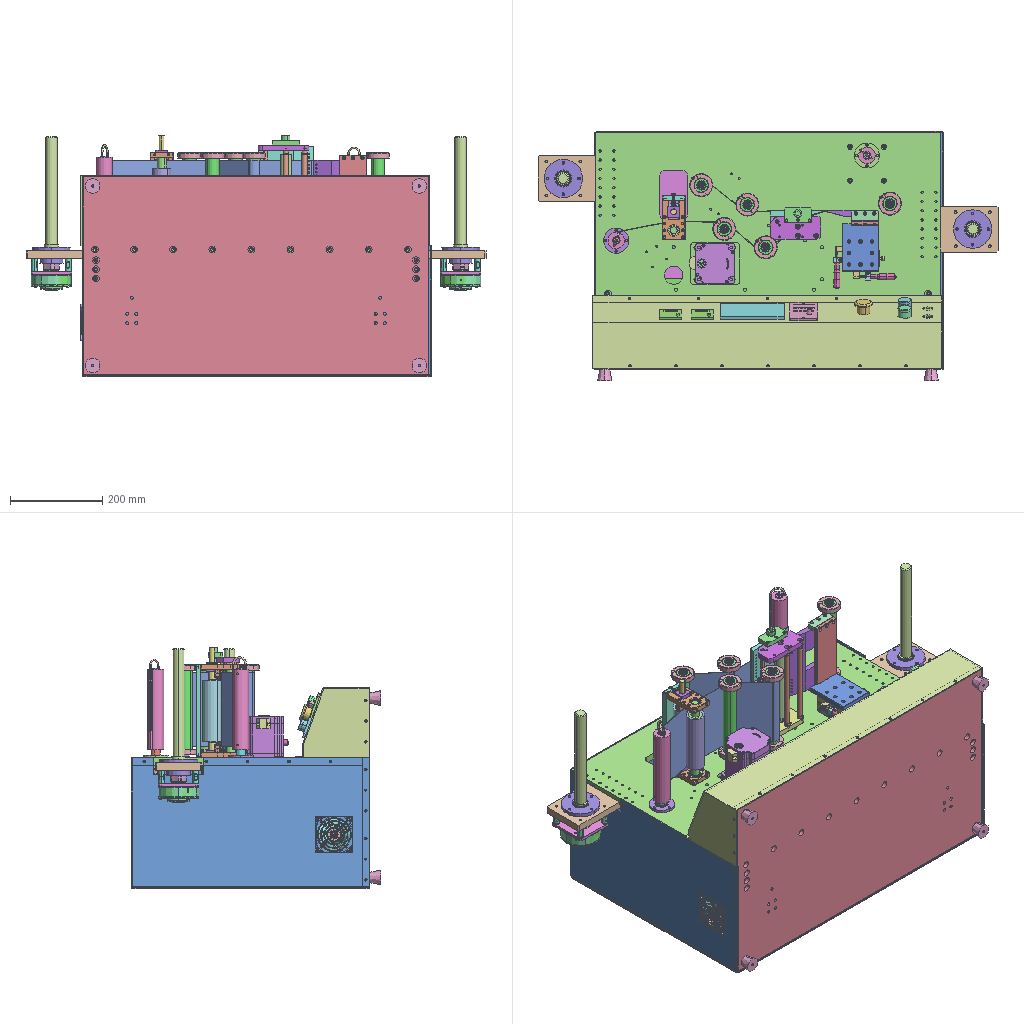Assembly | STEP file | 114 different items | 209 placed | box 1000 x 542 x 526 mm
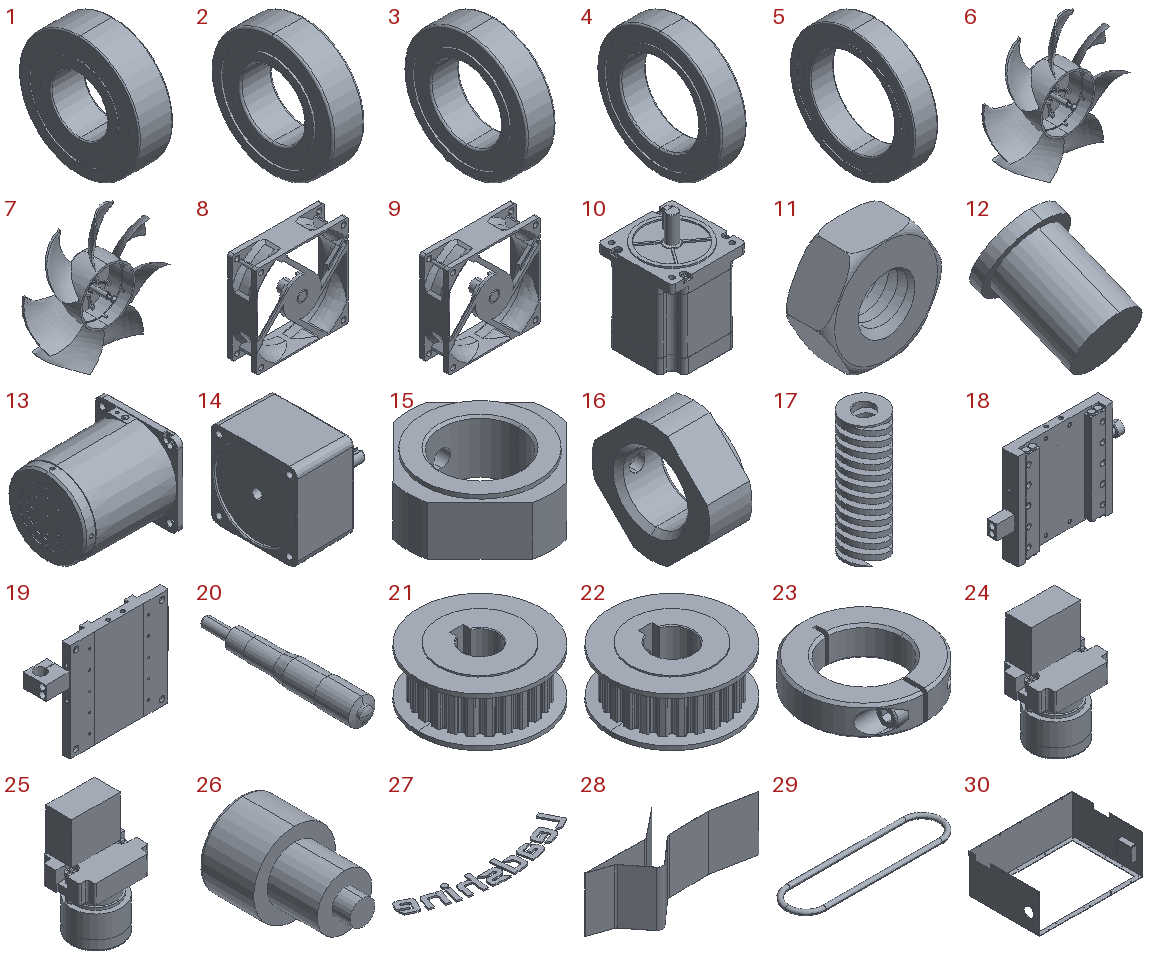Parts list (item | name | quantity | parent item | size | volume):
1 | 6002ZZ_Rolling bearings 6002 GB 276-94 | x2 | in Mirror MR-JDJ-G9 | 9 x 32 x 32 mm | 4596 mm3
2 | 61800ZZ_Rolling bearings 61800 GB 276-94 | x2 | in Mirror MR-JDJ-G6 | 5 x 19 x 19 mm | 823.307 mm3
3 | 61801ZZ_Rolling bearings 61801 GB 276-94 | x12 | in Mirror MR-JDJ-G11, Mirror MR-JDJ-G6 | 5 x 21 x 21 mm | 933.169 mm3
4 | 61802ZZ_Rolling bearings 61802 GB 276-94 | x2 | in Mirror MR-JDJ-G9 | 5 x 24 x 24 mm | 1110 mm3
5 | 61805ZZ_Rolling bearings 61805 GB 276-94 | x2 | in Mirror MR-JDJ-G7 | 7 x 37 x 37 mm | 3206 mm3
6 | 8025RYE_3_1 | x1 | - | 74.924 x 20.1 x 75 mm | 5435 mm3
7 | 8025RYE_3_1.stp | x1 | - | 74.924 x 20.1 x 75 mm | 5427 mm3
8 | 8025R_9_1 | x1 | - | 80 x 25 x 80 mm | 22604 mm3
9 | 8025R_9_1.stp | x1 | - | 80 x 25 x 80 mm | 22585 mm3
10 | 86CM45_1 | x1 | in 3D_Model_upload_86CM80 | 86 x 86 x 130 mm | 655714 mm3
11 | AD-3MM-2_1_2.stp | x1 | in ZHB01_ASM_1_ASM.stp | - | 44.135 mm3
12 | ADMI9201SOYF_11_1 | x1 | in ADMI9201SOYF_ASM_1_ASM | 13 x 18.798 x 16.741 mm | 788.076 mm3
13 | ADMI9201SOYF_22_1 | x1 | in ADMI9201SOYF_ASM_1_ASM | 142 x 90 x 90 mm | 645514 mm3
14 | ADMI9201SOYF_24_1_1 | x1 | in ADMI9201SOYF_ASM_1_1_ASM | 92 x 90 x 90 mm | 446981 mm3
15 | BKN26-M20 | x1 | in MR-JDJ-G | 35 x 35 x 13 mm | 6926 mm3
16 | BNG16 | x2 | in MR-JDJ-G, MR-JDJ-G2 | 10 x 25 x 25 mm | 2769 mm3
17 | - | x1 | in MR-JDJ-G | 10 x 10 x 30 mm | 930.907 mm3
18 | E-EIC31-80-001 | x2 | in E-EIC31-80 | 107.5 x 13 x 80 mm | 58649 mm3
19 | E-EIC31-80-002 | x2 | in E-EIC31-80 | 99.5 x 19 x 80 mm | 49389 mm3
20 | E-EIC31-80-003 | x2 | in E-EIC31-80 | 13 x 80.5 x 13 mm | 6930 mm3
21 | EAF51-XL050-24-A-N-d12_7 | x1 | in MR-JDJ-G | 45 x 45 x 19 mm | 19278 mm3
22 | EAF51-XL050-24-A-N-d15 | x1 | in MR-JDJ-G | 45 x 45 x 19 mm | 18328 mm3
23 | FAF06-D30 | x10 | in Mirror MR-JDJ-G11 | 50 x 49.989 x 12 mm | 14205 mm3
24 | Flat head illuminated push button (green) | x1 | in MR-JDJ-G | 40 x 30 x 63 mm | 37927 mm3
25 | Flat round head push button (yellow) | x1 | in MR-JDJ-G | 40 x 30 x 63 mm | 37927 mm3
26 | Hex socket bolt M12x10 | x1 | in MR-JDJ-G | 18 x 27 x 18 mm | 3856 mm3
27 | LOGO123_1 | x2 | in 3D_Model_upload_86CM80 | 23.395 x 5.753 x 0.2 mm | 6.476 mm3
28 | Layout^ | x1 | in MR-JDJ-G | 459.008 x 163.495 x 160 mm | 64878 mm3
29 | MBT5-380 | x1 | in MR-JDJ-G | 172.168 x 45 x 5 mm | 7461 mm3
30 | MT-COMBO-119-S001_Default<Machined> | x1 | in Sheet metal cover^ | 758 x 516.5 x 282.5 mm | 1425060 mm3
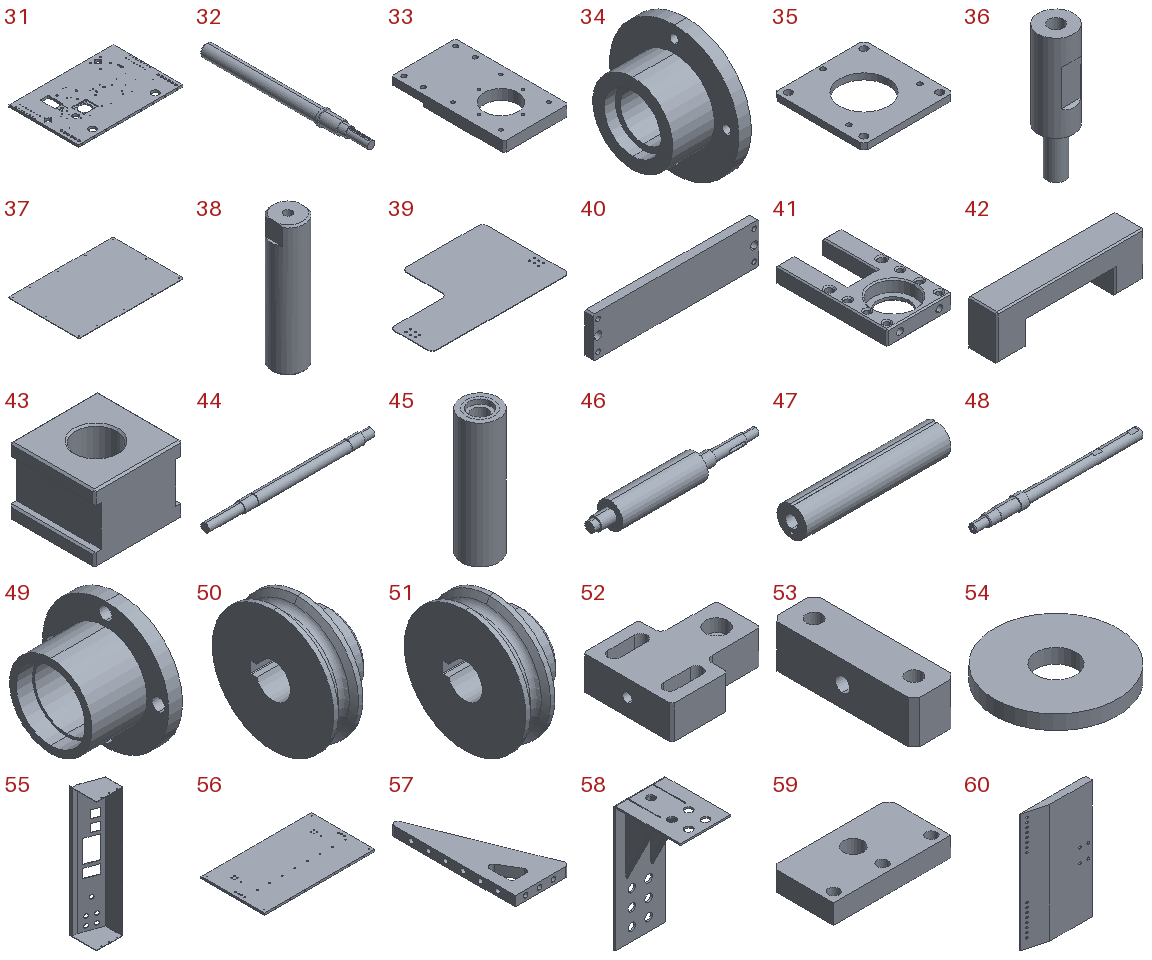31 | MT-COMBO-119-S002 | x1 | in MR-JDJ-G | 750 x 500 x 16 mm | 5589140 mm3
32 | MT-COMBO-119-S003 | x2 | in Mirror MR-JDJ-G7 | 30 x 334 x 30 mm | 147852 mm3
33 | MT-COMBO-119-S004 | x2 | in Mirror MR-JDJ-G7 | 100 x 175 x 16 mm | 217129 mm3
34 | MT-COMBO-119-S005 | x2 | in Mirror MR-JDJ-G7 | 35 x 84 x 84 mm | 71017 mm3
35 | MT-COMBO-119-S006 | x2 | in Mirror MR-JDJ-G7 | 88 x 88 x 6 mm | 34736 mm3
36 | MT-COMBO-119-S007_Default | x8 | in Mirror MR-JDJ-G7 | 12 x 12 x 44 mm | 3285 mm3
37 | MT-COMBO-119-S008 | x1 | in Sheet metal cover^ | 758 x 516.5 x 2.5 mm | 977840 mm3
38 | MT-COMBO-119-S009 | x4 | in MR-JDJ-G | 20 x 20 x 80 mm | 24237 mm3
39 | MT-COMBO-119-S010 | x1 | in MR-JDJ-G | 600 x 380 x 2 mm | 357256 mm3
40 | MT-COMBO-119-S011 | x1 | in Mirror MR-JDJ-G9 | 204 x 10 x 50 mm | 98448 mm3
41 | MT-COMBO-119-S012 | x2 | in Mirror MR-JDJ-G9 | 50 x 85 x 12 mm | 28835 mm3
42 | MT-COMBO-119-S013 | x2 | in Mirror MR-JDJ-G9 | 50 x 10 x 15 mm | 4828 mm3
43 | MT-COMBO-119-S014 | x2 | in Mirror MR-JDJ-G9 | 26 x 25 x 20 mm | 9252 mm3
44 | MT-COMBO-119-S015 | x1 | in Mirror MR-JDJ-G9 | 239 x 15 x 15 mm | 37577 mm3
45 | MT-COMBO-119-S016 | x1 | in Mirror MR-JDJ-G9 | 40 x 40 x 134 mm | 135720 mm3
46 | MT-COMBO-119-S017 | x1 | in Mirror MR-JDJ-G9 | 260 x 40 x 40 mm | 195020 mm3
47 | MT-COMBO-119-S018 | x2 | in MR-JDJ-G, MR-JDJ-G2 | 175 x 36 x 35.889 mm | 143638 mm3
48 | MT-COMBO-119-S019 | x1 | in MR-JDJ-G2 | 252 x 20 x 20 mm | 45952 mm3
49 | MT-COMBO-119-S020 | x1 | in MR-JDJ-G2 | 30 x 55 x 55 mm | 18366 mm3
50 | MT-COMBO-119-S021 | x1 | in MR-JDJ-G2 | 20 x 42 x 42 mm | 14178 mm3
51 | MT-COMBO-119-S022 | x1 | in MR-JDJ-G | 20 x 42 x 42 mm | 14178 mm3
52 | MT-COMBO-119-S023 | x1 | in MR-JDJ-G3 | 50 x 40 x 15 mm | 18974 mm3
53 | MT-COMBO-119-S024 | x1 | in MR-JDJ-G3 | 15 x 50 x 15 mm | 10123 mm3
54 | MT-COMBO-119-S025 | x2 | in MR-JDJ-G2 | 17 x 17 x 2 mm | 406.444 mm3
55 | MT-COMBO-119-S026 | x1 | in Sheet metal cover^ | 152.5 x 160 x 758 mm | 557156 mm3
56 | MT-COMBO-119-S027 | x1 | in MR-JDJ-G | 750 x 430 x 14 mm | 4475183 mm3
57 | MT-COMBO-119-S028 | x2 | in MR-JDJ-G | 77.615 x 179.037 x 14 mm | 94866 mm3
58 | MT-COMBO-119-S029 | x2 | in MR-JDJ-G | 60 x 80 x 150 mm | 38097 mm3
59 | MT-COMBO-119-S030 | x1 | in Mirror MR-JDJ-G6 | 60 x 32 x 10 mm | 17580 mm3
60 | MT-COMBO-119-S031 | x1 | in Mirror MR-JDJ-G6 | 120 x 12 x 215 mm | 252530 mm3
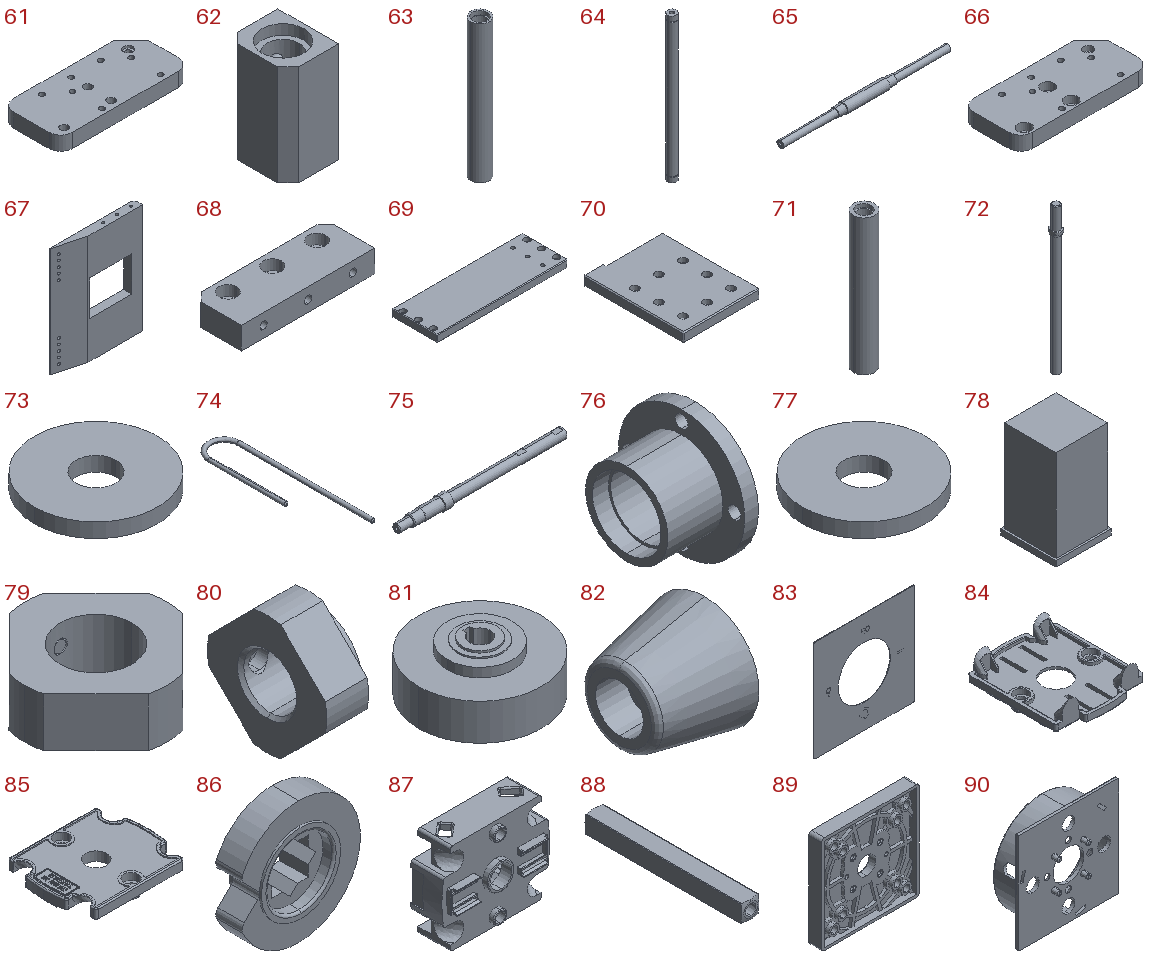61 | MT-COMBO-119-S032 | x1 | in Mirror MR-JDJ-G6 | 110 x 50 x 12 mm | 59904 mm3
62 | MT-COMBO-119-S033 | x1 | in Mirror MR-JDJ-G6 | 25 x 30 x 50 mm | 24424 mm3
63 | MT-COMBO-119-S034 | x1 | in Mirror MR-JDJ-G6 | 24 x 24 x 180 mm | 40008 mm3
64 | MT-COMBO-119-S035 | x3 | in Mirror MR-JDJ-G6 | 12 x 12 x 195 mm | 21406 mm3
65 | MT-COMBO-119-S036 | x1 | in Mirror MR-JDJ-G6 | 199 x 12 x 12 mm | 13503 mm3
66 | MT-COMBO-119-S037 | x1 | in Mirror MR-JDJ-G6 | 110 x 50 x 12 mm | 59904 mm3
67 | MT-COMBO-119-S038 | x1 | in Assembly 2^ | 120 x 12 x 155 mm | 147093 mm3
68 | MT-COMBO-119-S039 | x2 | in Assembly 2^ | 60 x 22 x 10 mm | 11821 mm3
69 | MT-COMBO-119-S040 | x1 | in Assembly 2^ | 175 x 60 x 10 mm | 101899 mm3
70 | MT-COMBO-119-S041 | x1 | in Assembly 2^ | 80 x 103 x 10 mm | 77497 mm3
71 | MT-COMBO-119-S042 | x5 | in Mirror MR-JDJ-G11 | 30 x 30 x 195 mm | 87297 mm3
72 | MT-COMBO-119-S043 | x5 | in Mirror MR-JDJ-G11 | 14 x 18 x 237 mm | 27010 mm3
73 | MT-COMBO-119-S044 | x5 | in Mirror MR-JDJ-G11 | 17 x 17 x 2 mm | 406.444 mm3
74 | MT-COMBO-119-S045 | x2 | in MR-JDJ-G, MR-JDJ-G2 | 34 x 157 x 4 mm | 3346 mm3
75 | MT-COMBO-119-S046 | x1 | in MR-JDJ-G | 252 x 20 x 20 mm | 45952 mm3
76 | MT-COMBO-119-S047 | x1 | in MR-JDJ-G | 30 x 55 x 55 mm | 18366 mm3
77 | MT-COMBO-119-S048 | x1 | in MR-JDJ-G | 17 x 17 x 2 mm | 406.444 mm3
78 | Magnetic powder tension controller | x2 | in MR-JDJ-G | 48 x 48 x 90 mm | 173670 mm3
79 | Mirror BNG20 | x2 | in Mirror MR-JDJ-G7 | 35 x 35 x 13 mm | 7455 mm3
80 | Mirror BNR10 | x2 | in Mirror MR-JDJ-G6 | 8 x 20 x 20 mm | 1587 mm3
81 | Mirror ZX3YN | x2 | in Mirror MR-JDJ-G7 | 88 x 88 x 44 mm | 175155 mm3
82 | NHY11-32 | x4 | in MR-JDJ-G | 25 x 32 x 32 mm | 12742 mm3
83 | PCS-01CC-2_1_2.stp | x1 | in ZHB01_ASM_1_ASM.stp | 62 x 0.3 x 62 mm | 908.364 mm3
84 | PCS-02B-3_1_2.stp | x1 | in ZHB01_ASM_1_ASM.stp | 38 x 45.04 x 11.674 mm | 2792 mm3
85 | PCS-02C2-3_1_2.stp | x1 | in ZHB01_ASM_1_ASM.stp | 45.039 x 38 x 7.5 mm | 4082 mm3
86 | PCS-04A-3_1_2.stp | x2 | in ZHB01_ASM_1_ASM.stp | 16.138 x 5.4 x 16.8 mm | 681.99 mm3
87 | PCS-11A-3_1_2.stp | x1 | in ZHB01_ASM_1_ASM.stp | 45 x 16.5 x 38 mm | 7553 mm3
88 | PCS-C17C-1-2_1_2.stp | x1 | in ZHB01_ASM_1_ASM.stp | 5 x 45.6 x 5 mm | 1100 mm3
89 | PCS-P01A-2_1_2.stp | x1 | in ZHB01_ASM_1_ASM.stp | 65 x 8.5 x 65 mm | 14701 mm3
90 | PCS-P01B-2_1_2.stp | x1 | in ZHB01_ASM_1_ASM.stp | 61.7 x 20.5 x 61.7 mm | 10976 mm3
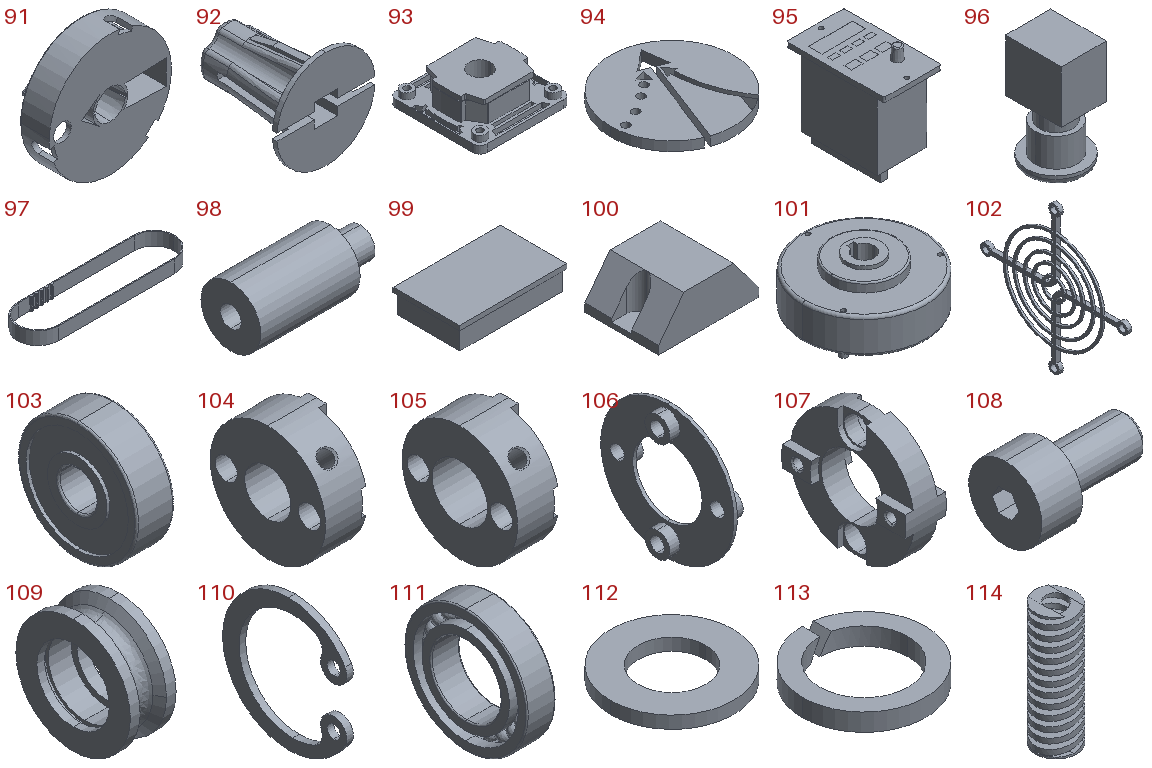91 | PCS-P05A-001-2_1_2.stp | x1 | in ZHB01_ASM_1_ASM.stp | 56 x 28.677 x 56 mm | 12848 mm3
92 | PCS-P06-2_1_2.stp | x1 | in ZHB01_ASM_1_ASM.stp | 20.946 x 21.8 x 21 mm | 1623 mm3
93 | PRT0120_3.stp | x1 | in ZHB01_ASM_1_ASM.stp | 60 x 60 x 20 mm | 35294 mm3
94 | Part 11_1 | x2 | in 3D_Model_upload_86CM80 | 16 x 16 x 1.2 mm | 213.852 mm3
95 | SF06E_Default | x1 | in MR-JDJ-G | 60 x 102 x 103.5 mm | 343869 mm3
96 | Stop button AS2201 | x1 | in MR-JDJ-G | 39 x 39 x 72 mm | 61878 mm3
97 | TBN138XL050_info-1-24-24 | x1 | in MR-JDJ-G | 154.6 x 40.3 x 12.7 mm | 4631 mm3
98 | Tension support column | x1 | in MR-JDJ-G3 | 26 x 12 x 12 mm | 2216 mm3
99 | Touch screen | x1 | in MR-JDJ-G | 139 x 86 x 31 mm | 341049 mm3
100 | Wire clamp block | x1 | in 3D_Model_upload_86CM80 | 30 x 22 x 12.5 mm | 6136 mm3
101 | YHD-LZ-PBN-0.3KG-yhd | x2 | in Mirror MR-JDJ-G7 | 88 x 88 x 43 mm | 168276 mm3
102 | ZHJ45-80 | x1 | in MR-JDJ-G | 3.7 x 109.009 x 109.011 mm | 3461 mm3
103 | _B626ZZ | x1 | in MBG28-2.5 | 6 x 19 x 19 mm | 1391 mm3
104 | _DBA11-D25-d10-e12-001.stp | x1 | in DBA11-D25-d10-e12.stp | 10.6 x 25 x 25 mm | 3291 mm3
105 | _DBA11-D25-d10-e12-002.stp | x1 | in DBA11-D25-d10-e12.stp | 10.6 x 25 x 25 mm | 2996 mm3
106 | _DBA11-D25-d10-e12-003.stp | x2 | in DBA11-D25-d10-e12.stp | 4.2 x 24 x 24 mm | 265.19 mm3
107 | _DBA11-D25-d10-e12-004.stp | x1 | in DBA11-D25-d10-e12.stp | 7.8 x 24 x 24 mm | 1439 mm3
108 | _DBA11-D25-d10-e12-005.stp | x8 | in DBA11-D25-d10-e12.stp | 7.5 x 4.5 x 4.5 mm | 61.818 mm3
109 | _MBG28-2.5mb | x1 | in MBG28-2.5 | 12 x 30 x 30 mm | 3875 mm3
110 | _RTWN19 | x1 | in MBG28-2.5 | 1 x 18.839 x 20 mm | 110.311 mm3
111 | deep groove ball bearings gb_61903 | x4 | in MR-JDJ-G, MR-JDJ-G2 | 7 x 30 x 30 mm | 2481 mm3
112 | plain washers--product grade c gb_PreviewCfg | x5 | in Mirror MR-JDJ-G11 | 10 x 10 x 1 mm | 54.782 mm3
113 | spring lock washers--normal type gb_PreviewCfg | x5 | in Mirror MR-JDJ-G11 | 4.2 x 4.2 x 0.6 mm | 3.946 mm3
114 | - | x1 | in Mirror MR-JDJ-G9 | 10 x 10 x 30 mm | 930.907 mm3